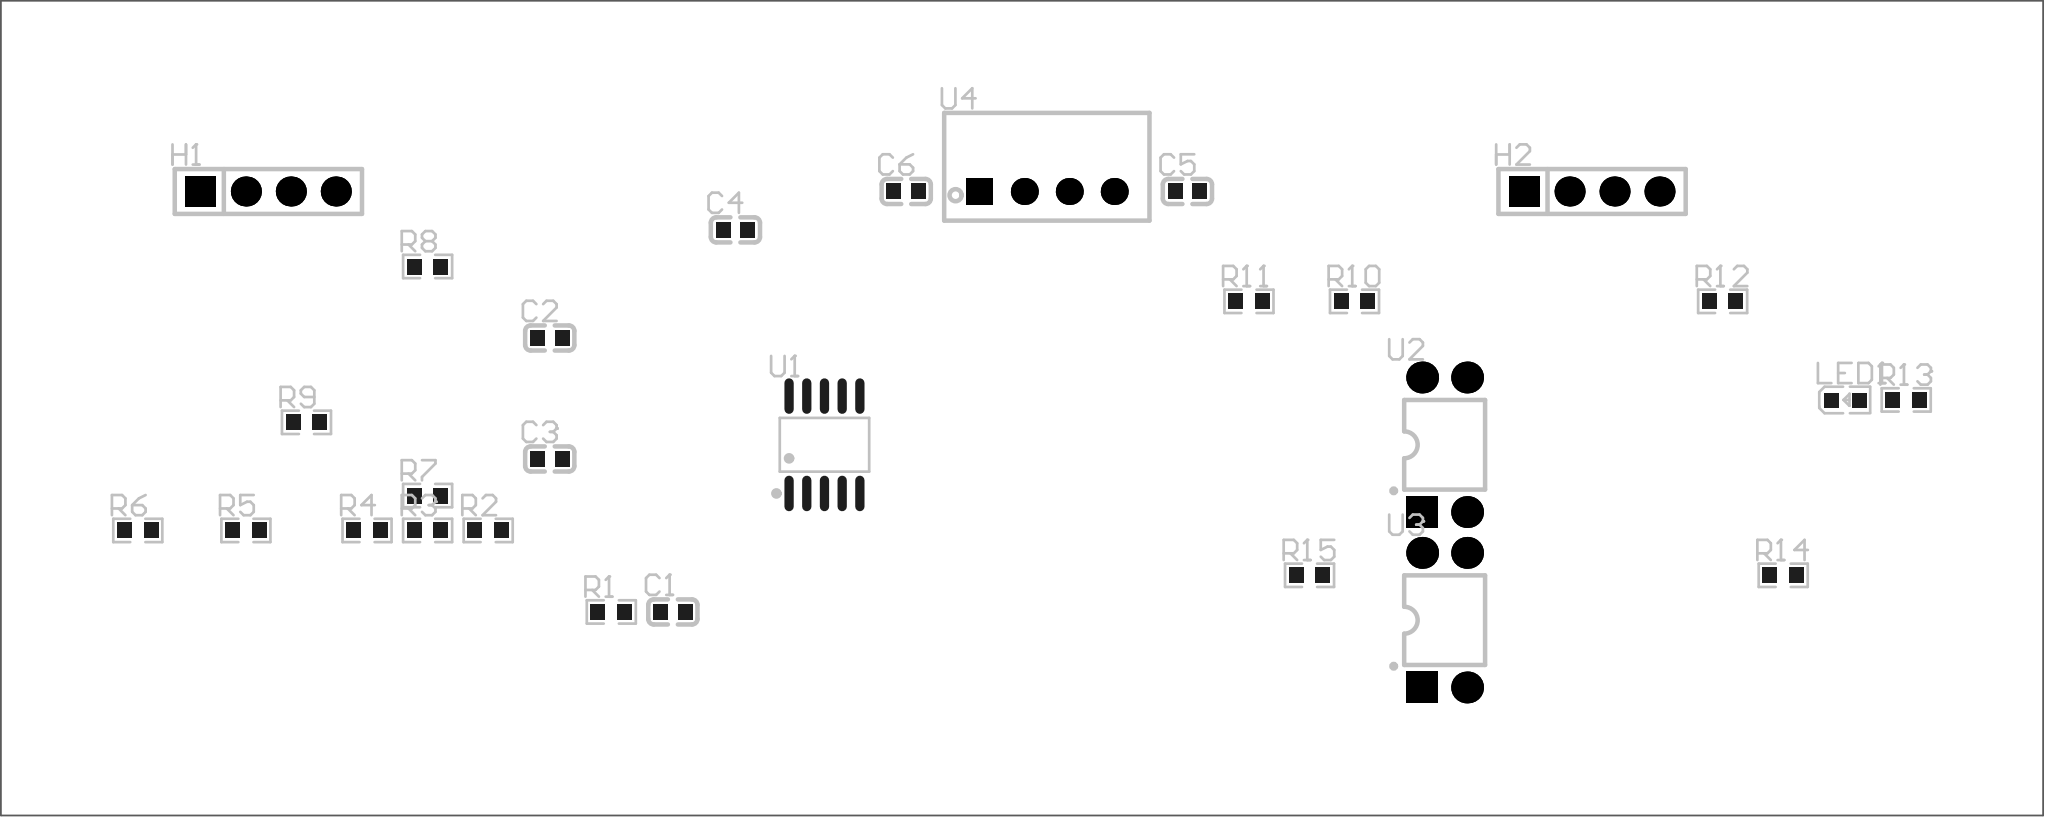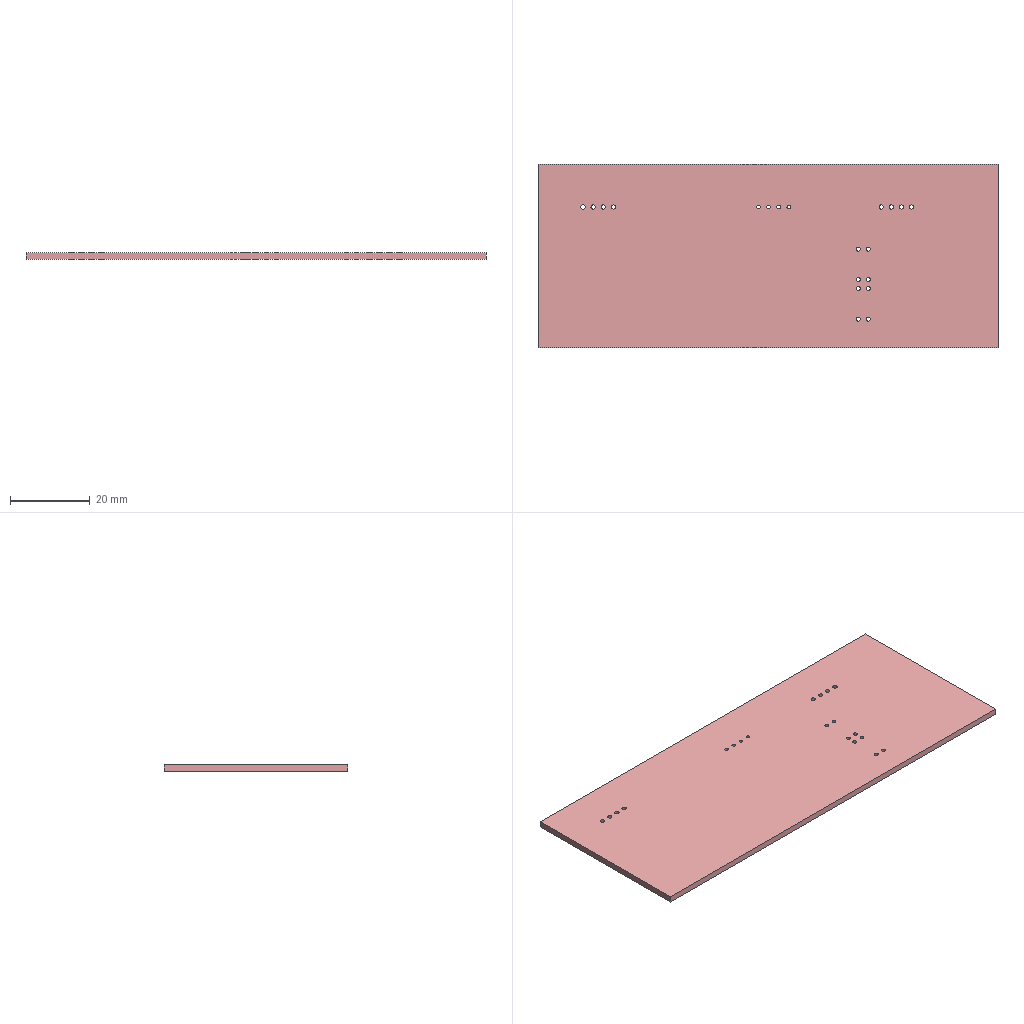Circuit board layout | Altium Designer | box 115.4 x 46.1 x 1.6 mm
Layer stack:
# Altium Designer layer stack of  (unit mm; dielectric type: 0 none, 1 core, 2 prepreg, 3 surface material)
index,name,kind,layer,copper_thickness_mm,dielectric_type,dielectric_thickness_mm,dielectric_material,dielectric_constant
0,Top Paste Mask Layer,other,,,,,,
1,Top Silkscreen Layer,other,,,,,,
2,Top Solder Mask Layer,dielectric,,,3,0.01,,3.3
3,Top Layer,copper,Top Layer,0.035,,,,
4,Dielectric1,dielectric,,,3,1.51,FR4,4.5
5,Bottom Layer,copper,Bottom Layer,0.035,,,,
6,Bottom Solder Mask Layer,dielectric,,,3,0.01,,3.3
7,Bottom Silkscreen Layer,other,,,,,,
8,Bottom Paste Mask Layer,other,,,,,,
# drill layer pairs: low layer,high layer
drill_pair,Top Layer,Bottom Layer
Part placement:
Designator,Comment,Layer,Footprint,Center-X(mm),Center-Y(mm),Rotation
C1,68nF,TopLayer,C0603,107.818,81.376,0
C2,68nF,TopLayer,C0603,100.862,96.888,0
C3,68nF,TopLayer,C0603,100.862,90.037,0
C4,100nF,TopLayer,C0603,111.352,103.01,0
C5,100nF,TopLayer,C0603,136.892,105.184,0
C6,100nF,TopLayer,C0603,121.004,105.184,0
H1,,TopLayer,HDR-TH_4P-P2.54-V-F,84.963,105.184,0
H2,,TopLayer,HDR-TH_4P-P2.54-V-F,159.755,105.184,0
LED1,,TopLayer,LED_0603,174.081,93.374,0
R1,510R,TopLayer,R0603,104.34,81.376,0
R2,390K,TopLayer,R0603,97.384,85.99,0
R3,390K,TopLayer,R0603,93.961,85.99,0
R4,390K,TopLayer,R0603,90.538,85.99,0
R5,390K,TopLayer,R0603,83.693,85.99,0
R6,390K,TopLayer,R0603,77.585,85.99,0
R7,510R,TopLayer,R0603,93.961,87.964,0
R8,510R,TopLayer,R0603,93.961,100.936,0
R9,510R,TopLayer,R0603,87.116,92.111,0
R10,1K,TopLayer,R0603,146.333,98.962,0
R11,10K,TopLayer,R0603,140.37,98.962,0
R12,3.3K,TopLayer,R0603,167.133,98.962,0
R13,3.3K,TopLayer,R0603,177.506,93.381,0
R14,10K,TopLayer,R0603,170.556,83.45,0
R15,1K,TopLayer,R0603,143.792,83.45,0
U1,BL0942,TopLayer,SSOP-10_L4.9-W3.9-P1.00-LS6.0-BL,116.384,90.841,0
U2,EL817B,TopLayer,DIP-4_L6.5-W4.6-P2.54-LS7.6-BL,151.425,90.841,0
U3,EL817B,TopLayer,DIP-4_L6.5-W4.6-P2.54-LS7.6-BL,151.425,80.91,0
U4,270kHz,TopLayer,PWRM-TH_B0305S-1WR2,128.948,105.184,0
Pad and via stacks:
# Altium Designer via and pad stacks of  (unit mm). Each distinct definition once, with the count of objects using it.
# via: kind,start_layer,end_layer,hole_mm,diameter_mm,mode(0 simple;1 top-mid-bottom;2 full stack),diameter_per_layer,count,example_net
# pad: kind,layer,hole_mm,hole_type(0 round;1 square;2 slot),plating,top_size,top_shape(1 round;2 rect;3 octagon;9 rounded rect),mid_size,bottom_size,mode,footprint,size_per_layer,count,example
pad,Top Layer,0,0,plated,0.8x0.9,2,0.8x0.9,0.8x0.9,0,C0603,,12,C1.2
pad,Top Layer,0,0,plated,0.8001x0.8001,2,0.8001x0.8001,0.8001x0.8001,0,LED_0603,,2,LED1.1
pad,Top Layer,0,0,plated,0.8065x0.864,2,0.8065x0.864,0.8065x0.864,0,R0603,,30,R1.2
pad,Top Layer,0,0,plated,0.525x2.014,1,0.525x2.014,0.525x2.014,0,SSOP-10_L4.9-W3.9-P1.00-LS6.0-BL,,10,U1.1
pad,Multi-Layer,1.1,0,plated,1.7x1.7,2,1.7x1.7,1.7x1.7,0,HDR-TH_4P-P2.54-V-F,,2,H1.1
pad,Multi-Layer,1.1,0,plated,1.7x1.7,1,1.7x1.7,1.7x1.7,0,HDR-TH_4P-P2.54-V-F,,6,H1.2
pad,Multi-Layer,1,0,plated,1.8x1.8,2,1.8x1.8,1.8x1.8,0,DIP-4_L6.5-W4.6-P2.54-LS7.6-BL,,2,U2.1
pad,Multi-Layer,1,0,plated,1.8x1.8,1,1.8x1.8,1.8x1.8,0,DIP-4_L6.5-W4.6-P2.54-LS7.6-BL,,6,U2.4
pad,Multi-Layer,0.9144,0,plated,1.524x1.524,1,1.524x1.524,1.524x1.524,0,PWRM-TH_B0305S-1WR2,,3,U4.4
pad,Multi-Layer,0.9144,0,plated,1.524x1.524,2,1.524x1.524,1.524x1.524,0,PWRM-TH_B0305S-1WR2,,1,U4.1
Design rules, without the lines most boards share:
# Altium Designer design rules of  (exported by Altium Designer, unit mm)
# columns: name | kind | enabled | priority | scope1 | scope2 | descriptor | typed fields (field=value)
creepage | 65 | enabled | 1 | All | All | Creepage Distance Constraint =(0mil) (All),(All) |